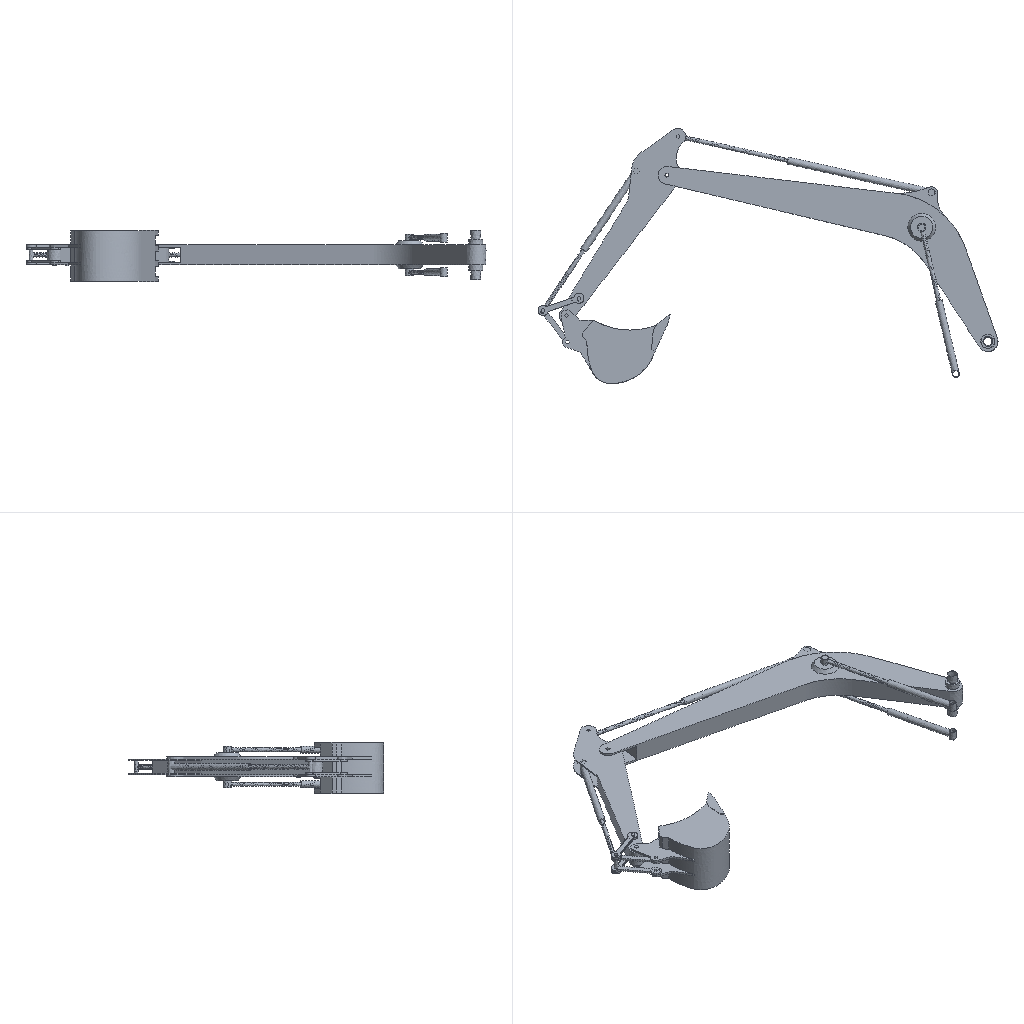Simulation study | ansys workbench
Set-up summary:
category,name,step,type,value,unit,region
solver,ansys_workbench
units,mm-N-s-tonne (MPa),,stated,"/units,MPA"
analysis,LS1,,static
load_step,LS1,LS1,static,nsubst=1; time=1
mesh,nodes,,,213522
mesh,elements,,,124253
element_type,SOLID187,,,108871
element_type,CONTA174,,,8886
element_type,SOLID186,,,5940
element_type,SURF154,,,556
material,Structural Steel,,E,200000,tonne s^-2 mm^-1
material,Structural Steel,,nu,0.3
material,Structural Steel,,density,7.85e-09,tonne mm^-3
material,Structural Steel,,conductivity,60.5,tonne mm s^-3 C^-1
material,Structural Steel,,specific_heat,4.34e+08,mm^2 s^-2 C^-1
material,Structural Steel,,cte,1.2e-05,C^-1
material,Structural Steel,,permeability,10000
material,Structural Steel,,resistivity,0.00017,ohm mm
load,Define Force Using Surface Effect Elements,LS1,surface-effect pres face 2,-0.325,,SURF154 #125
bc,"Create Joint ""? - ? ? Geom\1""",model,fixed,[dofs=ALL],,node list
contact,contact 1,,bonded (always),element=CONTA174
contact,contact 2,,bonded (always),element=CONTA174
contact,contact 3,,bonded (always),element=CONTA174
contact,contact 4,,bonded (always),element=CONTA174
contact,contact 5,,bonded (always),element=CONTA174
contact,contact 6,,bonded (always),element=CONTA174
contact,contact 7,,bonded (always),element=CONTA174
contact,contact 8,,bonded (always),element=CONTA174
contact,contact 9,,bonded (always),element=CONTA174
contact,contact 10,,bonded (always),element=CONTA174
contact,contact 11,,bonded (always),element=CONTA174
contact,contact 12,,bonded (always),element=CONTA174
contact,contact 13,,bonded (always),element=CONTA174
contact,contact 14,,bonded (always),element=CONTA174
contact,contact 15,,bonded (always),element=CONTA174
contact,contact 16,,bonded (always),element=CONTA174
contact,contact 17,,bonded (always),element=CONTA174
contact,contact 18,,bonded (always),element=CONTA174
contact,contact 19,,bonded (always),element=CONTA174
contact,contact 20,,bonded (always),element=CONTA174
contact,contact 21,,bonded (always),element=CONTA174
contact,contact 22,,bonded (always),element=CONTA174
contact,contact 23,,bonded (always),element=CONTA174
contact,contact 24,,bonded (always),element=CONTA174
contact,contact 25,,bonded (always),element=CONTA174
contact,contact 26,,bonded (always),element=CONTA174
contact,contact 27,,bonded (always),element=CONTA174
contact,contact 28,,bonded (always),element=CONTA174
contact,contact 29,,bonded (always),element=CONTA174
contact,contact 30,,bonded (always),element=CONTA174
contact,contact 31,,bonded (always),element=CONTA174
contact,contact 32,,bonded (always),element=CONTA174
contact,contact 33,,bonded (always),element=CONTA174
contact,contact 34,,bonded (always),element=CONTA174
contact,contact 35,,bonded (always),element=CONTA174
contact,contact 36,,bonded (always),element=CONTA174
contact,contact 37,,bonded (always),element=CONTA174
contact,contact 38,,bonded (always),element=CONTA174
contact,contact 39,,bonded (always),element=CONTA174
contact,contact 40,,bonded (always),element=CONTA174
contact,contact 41,,bonded (always),element=CONTA174
Ansys APDL input file, long lists of numbers shortened:
/batch
/config,noeldb,1     ! force off writing results to database
*get,_wallstrt,active,,time,wall
! ANSYS input file written by Workbench version 2021 R2
! File used for geometry attach:
/title,wbnew--____ (B5)
! ****** Begin Custom Load Command Snippet ******
/COM, ACT Extensions:
/COM,     LSDYNA, 2021.1
/COM,
! ****** End   Custom Load Command Snippet ******
*DIM,_wb_ProjectScratch_dir,string,248
_wb_ProjectScratch_dir(1) = ''
*DIM,_wb_SolverFiles_dir,string,248
_wb_SolverFiles_dir(1) = ''
*DIM,_wb_userfiles_dir,string,248
_wb_userfiles_dir(1) = ''
/com,--- Data in consistent NMM units. See Solving Units in the help system for more information.
/units,MPA
/nopr
/wb,file,start              !  signify a WB generated input file
/prep7
! Turn off shape checking because checks already performed inside WB mesher.
! See help system for more information.
SHPP,OFF,,NOWARN
/nolist
etcon,set             ! allow ANSYS to choose best KEYOP's for 180x elements, resets any applicable keyopt to MAPDL defaults
/com,*********** Nodes for the whole assembly ***********
nblock,3,,234821
(1i9,3e20.9e3)
   184906    -6.263799338E+03     2.243783554E+03    -1.950000000E+02
! (213473 more lines like these left out)
-1
/com,*********** Nodes for all Remote Points ***********
nblock,3
(1i9,3e20.9e3)
   213475    -1.651561260E+01     2.442490654E-12     0.000000000E+00
! (47 more lines like these left out)
-1
/wb,elem,start            !  set before creation of elements
/com,*********** Elements for Body 1 "Geom\311" ***********
et,1,187
eblock,19,solid,,54215
(19i9)
        1        1        1        1        0        0        0        0       10        0        1     5898     8234    11509     9197    51269    66550    51272    51271
! (108429 more lines like these left out)
-1
/com,*********** Elements for Body 2 "Geom\1" ***********
/com,*********** Send Body as a Rigid Body ***********
et,2,21
keyo,2,2,1             ! Moments of inertia in nodal coordinates
keyo,2,3,0         ! 3D Mass With Rotary Intertia
r,2,28.702,28.702,28.702,30418010.433,60387128.058,34538729.026
local,11,0,-33.672,530.917,-2.24517609878909e-004,-0.1259,2.91486308902519e-006,2.97554151848029e-006
nrot,81757
csys,0
mat,2
real,2
type,2
en,154848,81757
/com,*********** Elements for Body 3 "Geom\8112" ***********
et,3,187
eblock,19,solid,,16251
(19i9)
        3        3        3        3        0        0        0        0       10        0    54216    84875    85614    85045    85219   105120   106188   105115   105116
! (32501 more lines like these left out)
-1
/com,*********** Elements for Body 4 "Geom\9" ***********
et,4,187
eblock,19,solid,,6254
(19i9)
        4        4        4        4        0        0        0        0       10        0    70467   108116   109195   109196   109855   111675   117942   111676   111677
! (12507 more lines like these left out)
-1
/com,*********** Elements for Body 5 "Geom\10" ***********
et,5,187
eblock,19,solid,,3185
(19i9)
        5        5        5        5        0        0        0        0       10        0    76721   120466   120477   121060   120896   123279   123349   123282   123280
! (6369 more lines like these left out)
-1
! (12 more sections like these left out)
/com,*********** Send Body as a Rigid Body ***********
et,17,21
keyo,17,2,1             ! Moments of inertia in nodal coordinates
keyo,17,3,0         ! 3D Mass With Rotary Intertia
r,17,67.357,67.357,67.357,34318553.809,108925764.068,99398838.184
local,11,0,275.844,1783.618,105.607,-6.974,-7.686,22.634
nrot,213474
csys,0
mat,17
real,17
type,17
en,154849,213474
/wb,elem,end               !  done creating elements
/com,*********** Send User Defined Coordinate System(s) ***********
local,12,0,-16.516,2.44249065417534e-012,0.,0.,90.,0.
local,13,0,-7.10393372045205e-016,1049.,-4.43007760598127e-015,0.,-90.,0.
local,14,0,-407.516,1652.642,-330.,0.,0.,0.
local,15,0,-865.,1190.,-577.5,-180.,0.,-180.
local,16,0,-865.,1190.,-82.5,-180.,0.,-180.
local,17,0,-1351.909,3279.862,-577.5,0.,0.,0.
local,18,0,-1351.909,3279.862,-82.5,-180.,0.,-180.
local,19,0,-1209.585,3777.409,-330.,0.,0.,0.
local,20,0,-4827.516,4577.642,-330.,0.,0.,0.
local,21,0,-4987.516,4022.642,-330.,0.,0.,0.
local,22,0,-5422.516,4077.642,-330.,0.,0.,0.
local,23,0,-6241.745,2267.642,-457.5,0.,0.,0.
local,24,0,-6241.745,2267.642,-202.5,0.,0.,0.
local,25,0,-6416.836,2022.642,-330.,-180.,0.,-180.
local,26,0,-6401.836,1642.642,-457.5,0.,0.,0.
local,27,0,-6401.836,1642.642,-202.5,0.,0.,0.
local,28,0,-6751.836,2092.642,-457.5,0.,0.,0.
local,29,0,-6751.836,2092.642,-427.5,0.,0.,0.
local,30,0,-6751.836,2092.642,-202.5,0.,0.,0.
local,31,0,-6751.836,2092.642,-232.5,0.,0.,0.
local,32,0,-997.845,1760.185,-577.5,-76.885,0.,180.
local,33,0,-997.845,1760.185,-82.5,-76.885,0.,180.
local,34,0,-2249.452,4007.413,-330.,-12.472,0.,0.
local,35,0,-6396.31,2623.53,-330.,56.19,0.,0.
csys,0
toffst,273.15,  ! Temperature offset from absolute zero
/com,*********** Set Reference Temperature ***********
tref,22.
/wb,mat,start              !  starting to send materials
/com,*********** Send Materials ***********
Temperature = 'TEMP' ! Temperature
MP,DENS,1,7.85e-09,	! tonne mm^-3
MP,ALPX,1,1.2e-05,	! C^-1
MP,C,1,434000000,	! mm^2 s^-2 C^-1
MP,KXX,1,60.5,	! tonne mm s^-3 C^-1
MP,RSVX,1,0.00017,	! ohm mm
MP,EX,1,200000,	! tonne s^-2 mm^-1
MP,NUXY,1,0.3,
MP,MURX,1,10000,
Temperature = 'TEMP' ! Temperature
MP,DENS,2,7.85e-09,	! tonne mm^-3
MP,ALPX,2,1.2e-05,	! C^-1
MP,C,2,434000000,	! mm^2 s^-2 C^-1
MP,KXX,2,60.5,	! tonne mm s^-3 C^-1
MP,RSVX,2,0.00017,	! ohm mm
MP,EX,2,200000,	! tonne s^-2 mm^-1
MP,NUXY,2,0.3,
MP,MURX,2,10000,
Temperature = 'TEMP' ! Temperature
MP,DENS,3,7.85e-09,	! tonne mm^-3
MP,ALPX,3,1.2e-05,	! C^-1
MP,C,3,434000000,	! mm^2 s^-2 C^-1
MP,KXX,3,60.5,	! tonne mm s^-3 C^-1
MP,RSVX,3,0.00017,	! ohm mm
MP,EX,3,200000,	! tonne s^-2 mm^-1
MP,NUXY,3,0.3,
MP,MURX,3,10000,
Temperature = 'TEMP' ! Temperature
MP,DENS,4,7.85e-09,	! tonne mm^-3
MP,ALPX,4,1.2e-05,	! C^-1
MP,C,4,434000000,	! mm^2 s^-2 C^-1
MP,KXX,4,60.5,	! tonne mm s^-3 C^-1
MP,RSVX,4,0.00017,	! ohm mm
MP,EX,4,200000,	! tonne s^-2 mm^-1
MP,NUXY,4,0.3,
MP,MURX,4,10000,
Temperature = 'TEMP' ! Temperature
MP,DENS,5,7.85e-09,	! tonne mm^-3
MP,ALPX,5,1.2e-05,	! C^-1
MP,C,5,434000000,	! mm^2 s^-2 C^-1
MP,KXX,5,60.5,	! tonne mm s^-3 C^-1
MP,RSVX,5,0.00017,	! ohm mm
MP,EX,5,200000,	! tonne s^-2 mm^-1
MP,NUXY,5,0.3,
MP,MURX,5,10000,
Temperature = 'TEMP' ! Temperature
MP,DENS,6,7.85e-09,	! tonne mm^-3
MP,ALPX,6,1.2e-05,	! C^-1
MP,C,6,434000000,	! mm^2 s^-2 C^-1
MP,KXX,6,60.5,	! tonne mm s^-3 C^-1
MP,RSVX,6,0.00017,	! ohm mm
MP,EX,6,200000,	! tonne s^-2 mm^-1
MP,NUXY,6,0.3,
MP,MURX,6,10000,
Temperature = 'TEMP' ! Temperature
MP,DENS,7,7.85e-09,	! tonne mm^-3
MP,ALPX,7,1.2e-05,	! C^-1
MP,C,7,434000000,	! mm^2 s^-2 C^-1
MP,KXX,7,60.5,	! tonne mm s^-3 C^-1
MP,RSVX,7,0.00017,	! ohm mm
MP,EX,7,200000,	! tonne s^-2 mm^-1
MP,NUXY,7,0.3,
MP,MURX,7,10000,
Temperature = 'TEMP' ! Temperature
MP,DENS,8,7.85e-09,	! tonne mm^-3
MP,ALPX,8,1.2e-05,	! C^-1
MP,C,8,434000000,	! mm^2 s^-2 C^-1
MP,KXX,8,60.5,	! tonne mm s^-3 C^-1
MP,RSVX,8,0.00017,	! ohm mm
MP,EX,8,200000,	! tonne s^-2 mm^-1
MP,NUXY,8,0.3,
MP,MURX,8,10000,
Temperature = 'TEMP' ! Temperature
MP,DENS,9,7.85e-09,	! tonne mm^-3
MP,ALPX,9,1.2e-05,	! C^-1
MP,C,9,434000000,	! mm^2 s^-2 C^-1
MP,KXX,9,60.5,	! tonne mm s^-3 C^-1
MP,RSVX,9,0.00017,	! ohm mm
MP,EX,9,200000,	! tonne s^-2 mm^-1
! (74 more lines like these left out)
/wb,mat,end                !  done sending materials
!************************* Model Summary ********************
!Geom\311,	结构钢,	matid,	1
!Geom\1,	结构钢,	matid,	2
!Geom\8112,	结构钢,	matid,	3
!Geom\9,	结构钢,	matid,	4
!Geom\10,	结构钢,	matid,	5
!Geom\111,	结构钢,	matid,	6
!Geom\17,	结构钢,	matid,	7
!Geom\18,	结构钢,	matid,	8
!Geom\7,	结构钢,	matid,	9
!Geom\5,	结构钢,	matid,	10
!Geom\6,	结构钢,	matid,	11
!Geom\4,	结构钢,	matid,	12
!Geom\14,	结构钢,	matid,	13
!Geom\15,	结构钢,	matid,	14
!Geom\12,	结构钢,	matid,	15
!Geom\13,	结构钢,	matid,	16
!Geom\24,	结构钢,	matid,	17
!************************* End Model Summary ********************
! get the diagonal of the bounding box. Needed later for other things
*get,_xmin,node,,mnloc,x
*get,_ymin,node,,mnloc,y
*get,_zmin,node,,mnloc,z
*get,_xmax,node,,mxloc,x
*get,_ymax,node,,mxloc,y
*get,_zmax,node,,mxloc,z
_ASMDIAG=(_xmax-_xmin)*(_xmax-_xmin)+(_ymax-_ymin)*(_ymax-_ymin)+(_zmax-_zmin)*(_zmax-_zmin)
_ASMDIAG=SQRT(_ASMDIAG)
/wb,contact,start          !  starting to send contact
/wb,contact,end            !  done creating contacts
/golist
/wb,load,start             !  starting to send loads
/com,*********** Create Remote Point "内部远程点 2" ***********
! -------- Remote Point Used by "固定的 - 接地 至 Geom\1" --------
! ********* Create Contact to Connect To Rigid Body Mass Node ***********
*set,tid,18
*set,cid,18
et,tid,170
keyo,tid,2,1           ! Set MPC target element and not fix pilot
keyo,tid,4,0           ! Create CE's for all DOFs
type,tid
mat ,cid
real,cid
tshape,pilo
en,154922,81757
tshape
! ********* End of Create Contact to Connect To Rigid Body Mass Node ***********
*set,_npilot,213476
_npilot171=_npilot
mat,18
real,18
type,18
en,154923,81757,213476
csys,12
nrot,213476
csys,0
/com,*********** Create Remote Point "内部远程点 3" ***********
! -------- Remote Point Used by "固定的 - Geom\1 至 Geom\24" --------
*set,_npilot,213477
_npilot177=_npilot
mat,18
real,18
type,18
en,154924,81757,213477
csys,13
nrot,213477
csys,0
/com,*********** Create Remote Point "内部远程点 4" ***********
! -------- Remote Point Used by "固定的 - Geom\1 至 Geom\24" --------
! ********* Create Contact to Connect To Rigid Body Mass Node ***********
*set,tid,19
*set,cid,19
et,tid,170
keyo,tid,2,1           ! Set MPC target element and not fix pilot
keyo,tid,4,0           ! Create CE's for all DOFs
type,tid
mat ,cid
real,cid
tshape,pilo
en,154925,213474
tshape
! ********* End of Create Contact to Connect To Rigid Body Mass Node ***********
*set,_npilot,213478
_npilot178=_npilot
mat,19
real,19
type,19
en,154926,213474,213478
csys,13
nrot,213478
csys,0
/com,*********** Create Remote Point "内部远程点 5" ***********
! -------- Remote Point Used by "回转 - Geom\24 至 Geom\311" --------
*set,_npilot,213479
_npilot186=_npilot
mat,19
real,19
type,19
en,154927,213474,213479
/com,*********** Create Remote Point "内部远程点 6" ***********
! -------- Remote Point Used by "回转 - Geom\24 至 Geom\311" --------
*set,tid,21
*set,cid,20
et,cid,174
et,tid,170
keyo,tid,2,1               ! Don't fix the pilot node
keyo,tid,4,111111
keyo,cid,12,5              ! Bonded Contact
keyo,cid,4,2               ! Rigid CERIG style load
keyo,cid,2,2               ! MPC style contact
eblock,10,,,120
(15i9)
   154928       20       20       20        0        2     4141     1342     1342    11524    19992     1342    11520
! (119 more lines like these left out)
-1
*set,_npilot,213480
_npilot187=_npilot
type,tid
mat ,cid
real,cid
tshape,pilo
en,155048,_npilot
tshape
! (42 more sections like these left out)
/com,*********** Create Joint "固定的 - 接地 至 Geom\1" ***********
d,213476,all                   ! body to ground Direct D
/com,*********** Create Joint "固定的 - Geom\1 至 Geom\24" ***********
! Joint Element Type Declaration and Definition using CONTACT
*set,tid,102
*set,cid,102
et,tid,170
keyo,tid,2,1           ! Set MPC target element and not fix pilot
keyo,tid,4,0           ! Create CE's for all DOFs
mat,cid
real,cid
type,tid
tshape,pilo
en,154851,213477        ! create pilot node for rigid link
tshape
type,cid
en,163857,213477,213478      ! body to body joint
csys,0
/com,*********** Create Joint "回转 - Geom\24 至 Geom\311" ***********
/com,            Real Constant Set For Above Joint Is 103
! Joint Element Type Declaration and Definition using MPC184
*set,_jid,103
et,_jid,184
keyo,_jid,1,6           ! Revolute Joint
keyo,_jid,4,1           ! Z Axis is revolute axis
sectype,_jid, joint, revo, _wbjoint
secjoint,,14,14
mat,_jid
real,_jid
type,_jid
secnum,_jid
en,154852,213479,213480      ! body to body joint
/com,*********** Create Joint "回转 - Geom\24 至 Geom\4" ***********
/com,            Real Constant Set For Above Joint Is 104
! Joint Element Type Declaration and Definition using MPC184
*set,_jid,104
et,_jid,184
keyo,_jid,1,6           ! Revolute Joint
keyo,_jid,4,1           ! Z Axis is revolute axis
sectype,_jid, joint, revo, _wbjoint
secjoint,,15,15
mat,_jid
real,_jid
type,_jid
secnum,_jid
en,154853,213481,213482      ! body to body joint
/com,*********** Create Joint "回转 - Geom\24 至 Geom\6" ***********
/com,            Real Constant Set For Above Joint Is 105
! Joint Element Type Declaration and Definition using MPC184
*set,_jid,105
et,_jid,184
keyo,_jid,1,6           ! Revolute Joint
keyo,_jid,4,1           ! Z Axis is revolute axis
sectype,_jid, joint, revo, _wbjoint
secjoint,,16,16
mat,_jid
real,_jid
type,_jid
secnum,_jid
en,154854,213483,213484      ! body to body joint
! (19 more sections like these left out)
/com,*********** Define Force Using Surface Effect Elements ***********
local,36,0,0.,0.,0.,0.,0.,0.
csys,0
et,125,154
eblock,10,,,556
(15i9)
   163858      125      125      125       36   126347   126346   127311   127311   132833   132839   127311   132848
! (555 more lines like these left out)
-1
esel,s,type,,125
keyop,125,2,1                ! Apply load in local coordinate system
keyop,125,7,1                ! Use original area so load is constant in large deformation
esel,all
/com,*********** Create Joint Drivers **********
/gst,on,on
fini
*get,_numnode,node,0,count
*get,_numelem,elem,0,count
*get, _MAXELEMNUM, elem, 0, NUM, MAX
*get, _MAXNODENUM, node, 0, NUM, MAX
*get, _MAXELEMTYPE, etyp, 0, NUM, MAX
*get, _MAXREALCONST, real, 0, NUM, MAX
/go
/wb,load,end               !  done creating loads
/com,--- Number of total nodes = %_numnode%
/com,--- Number of contact elements = 9442
/com,--- Number of spring elements = 0
/com,--- Number of bearing elements = 0
/com,--- Number of solid elements = 114813
/com,--- Number of condensed parts = 0
/com,--- Number of total elements = %_numelem%
*get,_wallbsol,active,,time,wall
/com,****************************************************************************
/com,*************************    SOLUTION       ********************************
/com,****************************************************************************
/solu
antype,0                   ! static analysis
_thickRatio=0.647   ! Ratio of thick parts in the model
eqsl,pcg,1e-8,,,,,,1
cntr,print,1               ! print out contact info and also make no initial contact an error
dmpoption,emat,no             ! Don't combine emat file for DANSYS
dmpoption,esav,no             ! Don't combine esav file for DANSYS
nldiag,cont,iter           ! print out contact info each equilibrium iteration
rescontrol,,none                 ! Do not keep any restart files
/com,****************************************************
/com,******************* SOLVE FOR LS 1 OF 1 ****************
esel,s,type,,125
nsle
sfe,all,1,pres,1,0.
sfe,all,2,pres,1,-0.325
sfe,all,3,pres,1,0.
nsel,all
esel,all
/nopr
/gopr
esel,s,type,,121
dj,all,ux,0.
esel,all
esel,s,type,,122
dj,all,ux,0.
esel,all
esel,s,type,,123
dj,all,ux,0.
esel,all
esel,s,type,,124
dj,all,ux,0.
esel,all
nsub,1,1,1
time,1.
outres,erase
outres,all,none
outres,nsol,all,
outres,rsol,all
outres,eangl,all
outres,etmp,all
outres,veng,all
outres,strs,all,
outres,epel,all,
outres,eppl,all,
outres,cont,all,
/nopr
esel,s,type,,2
esel,a,type,,17
esel,a,type,,103,124
cm,_elmisc,elem
esel,all
/gopr
outres,misc,all,_elmisc
! *********** WB SOLVE COMMAND ***********
! check interactive state
*get,ANSINTER_,active,,int
*if,ANSINTER_,ne,0,then
/eof
*endif
solve
/com *************** Write FE CONNECTORS *********
CEWRITE,file,ce,,INTE
/com,****************************************************
/com,*************** FINISHED SOLVE FOR LS 1 *************
*get,_wallasol,active,,time,wall
/nopr
*get,_numnode,node,0,count
*get,_numelem,elem,0,count
*get, _MAXELEMNUM, elem, 0, NUM, MAX
*get, _MAXNODENUM, node, 0, NUM, MAX,,,INTERNAL
*get, _MAXELEMTYPE, etyp, 0, NUM, MAX
*get, _MAXREALCONST, real, 0, NUM, MAX
/gopr
*get,_PCGITER,active,,solu,cgiter
/post1
xmlo,ENCODING,ISO-8859-1
xmlo,parm
/xml,parm,xml
fini
/gopr
*get,_walldone,active,,time,wall
_preptime=(_wallbsol-_wallstrt)*3600
_solvtime=(_wallasol-_wallbsol)*3600
_posttime=(_walldone-_wallasol)*3600
_totaltim=(_walldone-_wallstrt)*3600
*get,_dlbratio,active,0,solu,dlbr
*get,_combtime,active,0,solu,comb
*get,_ssmode,active,0,solu,ssmm
*get,_ndofs,active,0,solu,ndof
/com,--- Total number of nodes = %_numnode%
/com,--- Total number of elements = %_numelem%
/com,--- Element load balance ratio = %_dlbratio%
/com,--- Time to combine distributed files = %_combtime%
/com,--- Sparse memory mode = %_ssmode%
/com,--- Number of DOF = %_ndofs%
/wb,file,end               ! done with WB generated input
Results summary:
result,analyses[0].index,,,1
result,analyses[0].system,,,SYS
result,analyses[0].deck,,,deck.dat
result,analyses[0].solve_status,,,completed
result,analyses[0].analysis_type,,,static
result,analyses[0].physics,,,mechanical
result,analyses[0].unit_system,,,"NMM: mm, ton, N, s, mV, mA, degC"
result,analyses[0].n_sets,,,1
result,analyses[0].load_steps[0].set,set=1,,1
result,analyses[0].load_steps[0].time_or_freq,set=1,,1
result,analyses[0].load_steps[0].max_displacement_magnitude,set=1,,1.73813e+06
result,analyses[0].load_steps[0].max_von_mises_nodal,set=1,,439.933
result,analyses[0].load_steps[0].reaction_force_sum_xyz[1],set=1,,3.27668e+06
result,analyses[0].load_steps[0].reaction_force_sum_xyz[2],set=1,,200000
result,analyses[0].load_steps[0].reaction_force_sum_xyz[3],set=1,,-5.64523e-06
result,geometry_export[0][0],,,.step
result,geometry_export[0][1],,,ok
result,geometry_export[0][2],,,17